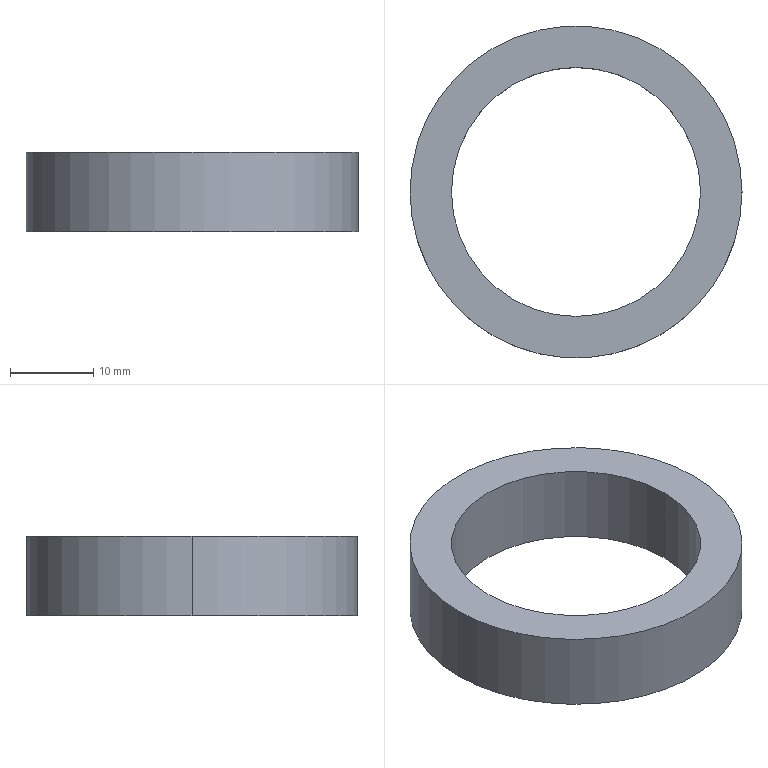Part | SolidWorks | features BaseBody 1 | 1 solid | 6 faces | box 40 x 40 x 9.581 mm | volume 5267 mm3 | cylinder 4 | plane 2 | commonest cylinder face diameters 30 x2 40 x2
STEP:
#1=CARTESIAN_POINT('',(15.,0.,9.581));
#2=VERTEX_POINT('',#1);
#3=CARTESIAN_POINT('',(-15.,0.,9.581));
#4=VERTEX_POINT('',#3);
#5=CARTESIAN_POINT('',(0.,0.,9.581));
#6=DIRECTION('',(0.,0.,-1.));
#7=DIRECTION('',(-1.,0.,0.));
#8=AXIS2_PLACEMENT_3D('',#5,#6,#7);
#9=CIRCLE('',#8,15.);
#10=EDGE_CURVE('',#2,#4,#9,.T.);
#11=ORIENTED_EDGE('',*,*,#10,.F.);
#12=CARTESIAN_POINT('',(15.,0.,0.));
#13=VERTEX_POINT('',#12);
#14=CARTESIAN_POINT('',(15.,0.,0.));
#15=DIRECTION('',(0.,0.,-1.));
#16=VECTOR('',#15,1000.);
#17=LINE('',#14,#16);
#18=EDGE_CURVE('',#2,#13,#17,.T.);
#19=ORIENTED_EDGE('',*,*,#18,.T.);
#20=CARTESIAN_POINT('',(-15.,0.,0.));
#21=VERTEX_POINT('',#20);
#22=CARTESIAN_POINT('',(0.,0.,0.));
#23=DIRECTION('',(0.,0.,1.));
#24=DIRECTION('',(-1.,0.,0.));
#25=AXIS2_PLACEMENT_3D('',#22,#23,#24);
#26=CIRCLE('',#25,15.);
#27=EDGE_CURVE('',#21,#13,#26,.T.);
#28=ORIENTED_EDGE('',*,*,#27,.F.);
#29=CARTESIAN_POINT('',(-15.,0.,0.));
#30=DIRECTION('',(0.,0.,-1.));
#31=VECTOR('',#30,1000.);
#32=LINE('',#29,#31);
#33=EDGE_CURVE('',#4,#21,#32,.T.);
#34=ORIENTED_EDGE('',*,*,#33,.F.);
#35=EDGE_LOOP('',(#11,#19,#28,#34));
#36=FACE_OUTER_BOUND('',#35,.T.);
#37=CARTESIAN_POINT('',(0.,0.,0.));
#38=DIRECTION('',(0.,0.,-1.));
#39=DIRECTION('',(-1.,0.,0.));
#40=AXIS2_PLACEMENT_3D('',#37,#38,#39);
#41=CYLINDRICAL_SURFACE('',#40,15.);
#42=ADVANCED_FACE('',(#36),#41,.F.);
#43=CARTESIAN_POINT('',(20.,0.,9.581));
#44=VERTEX_POINT('',#43);
#45=CARTESIAN_POINT('',(-20.,0.,9.581));
#46=VERTEX_POINT('',#45);
#47=CARTESIAN_POINT('',(0.,0.,9.581));
#48=DIRECTION('',(0.,0.,1.));
#49=DIRECTION('',(-1.,0.,0.));
#50=AXIS2_PLACEMENT_3D('',#47,#48,#49);
#51=CIRCLE('',#50,20.);
#52=EDGE_CURVE('',#44,#46,#51,.T.);
#53=ORIENTED_EDGE('',*,*,#52,.F.);
#54=CARTESIAN_POINT('',(20.,0.,0.));
#55=VERTEX_POINT('',#54);
#56=CARTESIAN_POINT('',(20.,0.,0.));
#57=DIRECTION('',(0.,0.,-1.));
#58=VECTOR('',#57,1000.);
#59=LINE('',#56,#58);
#60=EDGE_CURVE('',#44,#55,#59,.T.);
#61=ORIENTED_EDGE('',*,*,#60,.T.);
#62=CARTESIAN_POINT('',(-20.,0.,0.));
#63=VERTEX_POINT('',#62);
#64=CARTESIAN_POINT('',(0.,0.,0.));
#65=DIRECTION('',(0.,0.,-1.));
#66=DIRECTION('',(-1.,0.,0.));
#67=AXIS2_PLACEMENT_3D('',#64,#65,#66);
#68=CIRCLE('',#67,20.);
#69=EDGE_CURVE('',#63,#55,#68,.T.);
#70=ORIENTED_EDGE('',*,*,#69,.F.);
#71=CARTESIAN_POINT('',(-20.,0.,0.));
#72=DIRECTION('',(0.,0.,-1.));
#73=VECTOR('',#72,1000.);
#74=LINE('',#71,#73);
#75=EDGE_CURVE('',#46,#63,#74,.T.);
#76=ORIENTED_EDGE('',*,*,#75,.F.);
#77=EDGE_LOOP('',(#53,#61,#70,#76));
#78=FACE_OUTER_BOUND('',#77,.T.);
#79=CARTESIAN_POINT('',(0.,0.,0.));
#80=DIRECTION('',(0.,0.,-1.));
#81=DIRECTION('',(-1.,0.,0.));
#82=AXIS2_PLACEMENT_3D('',#79,#80,#81);
#83=CYLINDRICAL_SURFACE('',#82,20.);
#84=ADVANCED_FACE('',(#78),#83,.T.);
#85=ORIENTED_EDGE('',*,*,#27,.T.);
#86=CARTESIAN_POINT('',(0.,0.,0.));
#87=DIRECTION('',(0.,0.,1.));
#88=DIRECTION('',(-1.,0.,0.));
#89=AXIS2_PLACEMENT_3D('',#86,#87,#88);
#90=CIRCLE('',#89,15.);
#91=EDGE_CURVE('',#13,#21,#90,.T.);
#92=ORIENTED_EDGE('',*,*,#91,.T.);
#93=EDGE_LOOP('',(#85,#92));
#94=FACE_BOUND('',#93,.T.);
#95=ORIENTED_EDGE('',*,*,#69,.T.);
#96=CARTESIAN_POINT('',(0.,0.,0.));
#97=DIRECTION('',(0.,0.,-1.));
#98=DIRECTION('',(-1.,0.,0.));
#99=AXIS2_PLACEMENT_3D('',#96,#97,#98);
#100=CIRCLE('',#99,20.);
#101=EDGE_CURVE('',#55,#63,#100,.T.);
#102=ORIENTED_EDGE('',*,*,#101,.T.);
#103=EDGE_LOOP('',(#95,#102));
#104=FACE_OUTER_BOUND('',#103,.T.);
#105=CARTESIAN_POINT('',(0.,0.,0.));
#106=DIRECTION('',(0.,0.,1.));
#107=DIRECTION('',(1.,0.,0.));
#108=AXIS2_PLACEMENT_3D('',#105,#106,#107);
#109=PLANE('',#108);
#110=ADVANCED_FACE('',(#94,#104),#109,.F.);
#111=CARTESIAN_POINT('',(0.,0.,9.581));
#112=DIRECTION('',(0.,0.,-1.));
#113=DIRECTION('',(-1.,0.,0.));
#114=AXIS2_PLACEMENT_3D('',#111,#112,#113);
#115=CIRCLE('',#114,15.);
#116=EDGE_CURVE('',#4,#2,#115,.T.);
#117=ORIENTED_EDGE('',*,*,#116,.T.);
#118=ORIENTED_EDGE('',*,*,#10,.T.);
#119=EDGE_LOOP('',(#117,#118));
#120=FACE_BOUND('',#119,.T.);
#121=CARTESIAN_POINT('',(0.,0.,9.581));
#122=DIRECTION('',(0.,0.,1.));
#123=DIRECTION('',(-1.,0.,0.));
#124=AXIS2_PLACEMENT_3D('',#121,#122,#123);
#125=CIRCLE('',#124,20.);
#126=EDGE_CURVE('',#46,#44,#125,.T.);
#127=ORIENTED_EDGE('',*,*,#126,.T.);
#128=ORIENTED_EDGE('',*,*,#52,.T.);
#129=EDGE_LOOP('',(#127,#128));
#130=FACE_OUTER_BOUND('',#129,.T.);
#131=CARTESIAN_POINT('',(0.,0.,9.581));
#132=DIRECTION('',(0.,0.,1.));
#133=DIRECTION('',(1.,0.,0.));
#134=AXIS2_PLACEMENT_3D('',#131,#132,#133);
#135=PLANE('',#134);
#136=ADVANCED_FACE('',(#120,#130),#135,.T.);
#137=ORIENTED_EDGE('',*,*,#60,.F.);
#138=ORIENTED_EDGE('',*,*,#126,.F.);
#139=ORIENTED_EDGE('',*,*,#75,.T.);
#140=ORIENTED_EDGE('',*,*,#101,.F.);
#141=EDGE_LOOP('',(#137,#138,#139,#140));
#142=FACE_OUTER_BOUND('',#141,.T.);
#143=CARTESIAN_POINT('',(0.,0.,0.));
#144=DIRECTION('',(0.,0.,-1.));
#145=DIRECTION('',(-1.,0.,0.));
#146=AXIS2_PLACEMENT_3D('',#143,#144,#145);
#147=CYLINDRICAL_SURFACE('',#146,20.);
#148=ADVANCED_FACE('',(#142),#147,.T.);
#149=ORIENTED_EDGE('',*,*,#18,.F.);
#150=ORIENTED_EDGE('',*,*,#116,.F.);
#151=ORIENTED_EDGE('',*,*,#33,.T.);
#152=ORIENTED_EDGE('',*,*,#91,.F.);
#153=EDGE_LOOP('',(#149,#150,#151,#152));
#154=FACE_OUTER_BOUND('',#153,.T.);
#155=CARTESIAN_POINT('',(0.,0.,0.));
#156=DIRECTION('',(0.,0.,-1.));
#157=DIRECTION('',(-1.,0.,0.));
#158=AXIS2_PLACEMENT_3D('',#155,#156,#157);
#159=CYLINDRICAL_SURFACE('',#158,15.);
#160=ADVANCED_FACE('',(#154),#159,.F.);
#161=CLOSED_SHELL('',(#42,#84,#110,#136,#148,#160));
#162=MANIFOLD_SOLID_BREP('',#161);
#163=CARTESIAN_POINT('',(0.,0.,0.));
#164=DIRECTION('',(0.,0.,1.));
#165=DIRECTION('',(1.,0.,0.));
#166=AXIS2_PLACEMENT_3D('',#163,#164,#165);
#167=(LENGTH_UNIT()NAMED_UNIT(*)SI_UNIT(.MILLI.,.METRE.));
#168=UNCERTAINTY_MEASURE_WITH_UNIT(LENGTH_MEASURE(0.00001),#167,'','');
#169=(NAMED_UNIT(*)PLANE_ANGLE_UNIT()SI_UNIT($,.RADIAN.));
#170=(NAMED_UNIT(*)SI_UNIT($,.STERADIAN.)SOLID_ANGLE_UNIT());
#171=(GEOMETRIC_REPRESENTATION_CONTEXT(3)GLOBAL_UNCERTAINTY_ASSIGNED_CONTEXT((#168))GLOBAL_UNIT_ASSIGNED_CONTEXT((#167,#169,#170))REPRESENTATION_CONTEXT('',''));
#172=ADVANCED_BREP_SHAPE_REPRESENTATION('',(#162,#166),#171);